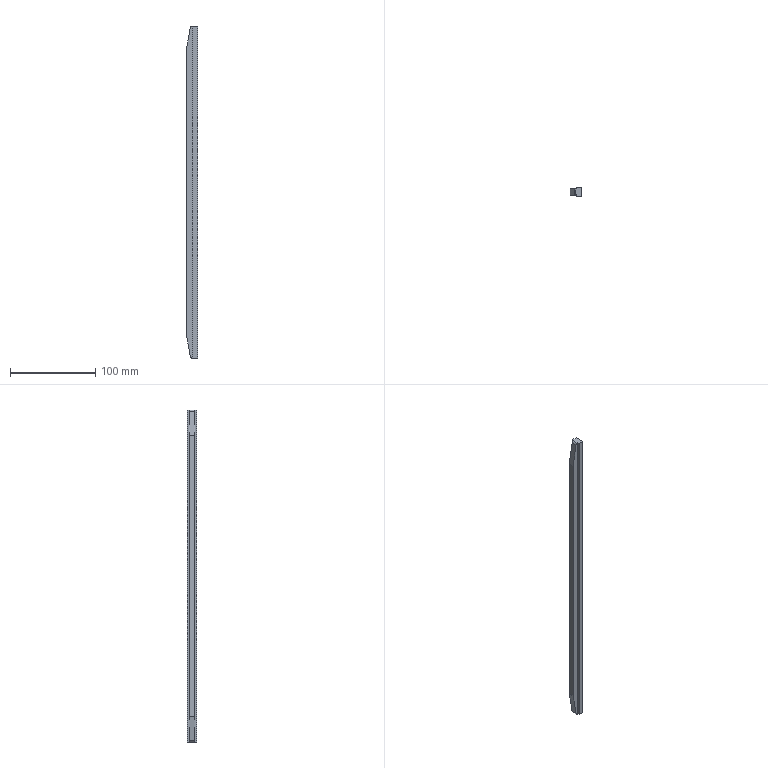Part | SolidWorks | features Chamfer 1, Extrusion 1, Fillet 1 | 1 solid | 16 faces | box 14 x 11 x 390 mm | volume 45277 mm3 | plane 12 | cylinder 4 | commonest cylinder face diameters 4 x4
STEP:
#1=CARTESIAN_POINT('',(0.,5.5,-195.));
#2=VERTEX_POINT('',#1);
#3=CARTESIAN_POINT('',(-6.,5.5,-195.));
#4=VERTEX_POINT('',#3);
#5=CARTESIAN_POINT('',(0.,5.5,-195.));
#6=DIRECTION('',(-1.,0.,0.));
#7=VECTOR('',#6,1000.);
#8=LINE('',#5,#7);
#9=EDGE_CURVE('',#2,#4,#8,.T.);
#10=ORIENTED_EDGE('',*,*,#9,.T.);
#11=CARTESIAN_POINT('',(-6.,5.5,195.));
#12=VERTEX_POINT('',#11);
#13=CARTESIAN_POINT('',(-6.,5.5,195.));
#14=DIRECTION('',(0.,0.,-1.));
#15=VECTOR('',#14,1000.);
#16=LINE('',#13,#15);
#17=EDGE_CURVE('',#12,#4,#16,.T.);
#18=ORIENTED_EDGE('',*,*,#17,.F.);
#19=CARTESIAN_POINT('',(0.,5.5,195.));
#20=VERTEX_POINT('',#19);
#21=CARTESIAN_POINT('',(0.,5.5,195.));
#22=DIRECTION('',(-1.,0.,0.));
#23=VECTOR('',#22,1000.);
#24=LINE('',#21,#23);
#25=EDGE_CURVE('',#20,#12,#24,.T.);
#26=ORIENTED_EDGE('',*,*,#25,.F.);
#27=CARTESIAN_POINT('',(0.,5.5,195.));
#28=DIRECTION('',(0.,0.,-1.));
#29=VECTOR('',#28,1000.);
#30=LINE('',#27,#29);
#31=EDGE_CURVE('',#20,#2,#30,.T.);
#32=ORIENTED_EDGE('',*,*,#31,.T.);
#33=EDGE_LOOP('',(#10,#18,#26,#32));
#34=FACE_OUTER_BOUND('',#33,.T.);
#35=CARTESIAN_POINT('',(0.,5.5,195.));
#36=DIRECTION('',(0.,-1.,0.));
#37=DIRECTION('',(1.,0.,0.));
#38=AXIS2_PLACEMENT_3D('',#35,#36,#37);
#39=PLANE('',#38);
#40=ADVANCED_FACE('',(#34),#39,.F.);
#41=CARTESIAN_POINT('',(-6.,3.3,-195.));
#42=VERTEX_POINT('',#41);
#43=CARTESIAN_POINT('',(-6.,5.5,-195.));
#44=DIRECTION('',(0.,-1.,0.));
#45=VECTOR('',#44,1000.);
#46=LINE('',#43,#45);
#47=EDGE_CURVE('',#4,#42,#46,.T.);
#48=ORIENTED_EDGE('',*,*,#47,.T.);
#49=CARTESIAN_POINT('',(-6.,3.3,195.));
#50=VERTEX_POINT('',#49);
#51=CARTESIAN_POINT('',(-6.,3.3,195.));
#52=DIRECTION('',(0.,0.,-1.));
#53=VECTOR('',#52,1000.);
#54=LINE('',#51,#53);
#55=EDGE_CURVE('',#50,#42,#54,.T.);
#56=ORIENTED_EDGE('',*,*,#55,.F.);
#57=CARTESIAN_POINT('',(-6.,5.5,195.));
#58=DIRECTION('',(0.,-1.,0.));
#59=VECTOR('',#58,1000.);
#60=LINE('',#57,#59);
#61=EDGE_CURVE('',#12,#50,#60,.T.);
#62=ORIENTED_EDGE('',*,*,#61,.F.);
#63=ORIENTED_EDGE('',*,*,#17,.T.);
#64=EDGE_LOOP('',(#48,#56,#62,#63));
#65=FACE_OUTER_BOUND('',#64,.T.);
#66=CARTESIAN_POINT('',(-6.,5.5,195.));
#67=DIRECTION('',(1.,0.,0.));
#68=DIRECTION('',(0.,0.,-1.));
#69=AXIS2_PLACEMENT_3D('',#66,#67,#68);
#70=PLANE('',#69);
#71=ADVANCED_FACE('',(#65),#70,.F.);
#72=CARTESIAN_POINT('',(-13.97,3.3,165.172));
#73=VERTEX_POINT('',#72);
#74=CARTESIAN_POINT('',(-9.002,3.3,193.347));
#75=VERTEX_POINT('',#74);
#76=CARTESIAN_POINT('',(-8.71,3.3,195.));
#77=DIRECTION('',(0.1736,0.,0.9848));
#78=VECTOR('',#77,1000.);
#79=LINE('',#76,#78);
#80=EDGE_CURVE('',#73,#75,#79,.T.);
#81=ORIENTED_EDGE('',*,*,#80,.T.);
#82=CARTESIAN_POINT('',(-7.032,3.3,195.));
#83=VERTEX_POINT('',#82);
#84=CARTESIAN_POINT('',(-7.032,3.3,193.));
#85=DIRECTION('',(0.,1.,0.));
#86=DIRECTION('',(1.,0.,0.));
#87=AXIS2_PLACEMENT_3D('',#84,#85,#86);
#88=CIRCLE('',#87,2.);
#89=EDGE_CURVE('',#75,#83,#88,.T.);
#90=ORIENTED_EDGE('',*,*,#89,.T.);
#91=CARTESIAN_POINT('',(-6.,3.3,195.));
#92=DIRECTION('',(-1.,0.,0.));
#93=VECTOR('',#92,1000.);
#94=LINE('',#91,#93);
#95=EDGE_CURVE('',#50,#83,#94,.T.);
#96=ORIENTED_EDGE('',*,*,#95,.F.);
#97=ORIENTED_EDGE('',*,*,#55,.T.);
#98=CARTESIAN_POINT('',(-7.032,3.3,-195.));
#99=VERTEX_POINT('',#98);
#100=CARTESIAN_POINT('',(-6.,3.3,-195.));
#101=DIRECTION('',(-1.,0.,0.));
#102=VECTOR('',#101,1000.);
#103=LINE('',#100,#102);
#104=EDGE_CURVE('',#42,#99,#103,.T.);
#105=ORIENTED_EDGE('',*,*,#104,.T.);
#106=CARTESIAN_POINT('',(-9.002,3.3,-193.347));
#107=VERTEX_POINT('',#106);
#108=CARTESIAN_POINT('',(-7.032,3.3,-193.));
#109=DIRECTION('',(0.,1.,0.));
#110=DIRECTION('',(1.,0.,0.));
#111=AXIS2_PLACEMENT_3D('',#108,#109,#110);
#112=CIRCLE('',#111,2.);
#113=EDGE_CURVE('',#99,#107,#112,.T.);
#114=ORIENTED_EDGE('',*,*,#113,.T.);
#115=CARTESIAN_POINT('',(-13.97,3.3,-165.172));
#116=VERTEX_POINT('',#115);
#117=CARTESIAN_POINT('',(-14.,3.3,-165.));
#118=DIRECTION('',(-0.1736,0.,0.9848));
#119=VECTOR('',#118,1000.);
#120=LINE('',#117,#119);
#121=EDGE_CURVE('',#107,#116,#120,.T.);
#122=ORIENTED_EDGE('',*,*,#121,.T.);
#123=CARTESIAN_POINT('',(-14.,3.3,-164.825));
#124=VERTEX_POINT('',#123);
#125=CARTESIAN_POINT('',(-12.,3.3,-164.825));
#126=DIRECTION('',(0.,1.,0.));
#127=DIRECTION('',(1.,0.,0.));
#128=AXIS2_PLACEMENT_3D('',#125,#126,#127);
#129=CIRCLE('',#128,2.);
#130=EDGE_CURVE('',#116,#124,#129,.T.);
#131=ORIENTED_EDGE('',*,*,#130,.T.);
#132=CARTESIAN_POINT('',(-14.,3.3,164.825));
#133=VERTEX_POINT('',#132);
#134=CARTESIAN_POINT('',(-14.,3.3,195.));
#135=DIRECTION('',(0.,0.,-1.));
#136=VECTOR('',#135,1000.);
#137=LINE('',#134,#136);
#138=EDGE_CURVE('',#133,#124,#137,.T.);
#139=ORIENTED_EDGE('',*,*,#138,.F.);
#140=CARTESIAN_POINT('',(-12.,3.3,164.825));
#141=DIRECTION('',(0.,1.,0.));
#142=DIRECTION('',(1.,0.,0.));
#143=AXIS2_PLACEMENT_3D('',#140,#141,#142);
#144=CIRCLE('',#143,2.);
#145=EDGE_CURVE('',#133,#73,#144,.T.);
#146=ORIENTED_EDGE('',*,*,#145,.T.);
#147=EDGE_LOOP('',(#81,#90,#96,#97,#105,#114,#122,#131,#139,#146));
#148=FACE_OUTER_BOUND('',#147,.T.);
#149=CARTESIAN_POINT('',(-6.,3.3,195.));
#150=DIRECTION('',(0.,-1.,0.));
#151=DIRECTION('',(1.,0.,0.));
#152=AXIS2_PLACEMENT_3D('',#149,#150,#151);
#153=PLANE('',#152);
#154=ADVANCED_FACE('',(#148),#153,.F.);
#155=CARTESIAN_POINT('',(-14.,-3.3,164.825));
#156=VERTEX_POINT('',#155);
#157=CARTESIAN_POINT('',(-14.,-3.3,-164.825));
#158=VERTEX_POINT('',#157);
#159=CARTESIAN_POINT('',(-14.,-3.3,195.));
#160=DIRECTION('',(0.,0.,-1.));
#161=VECTOR('',#160,1000.);
#162=LINE('',#159,#161);
#163=EDGE_CURVE('',#156,#158,#162,.T.);
#164=ORIENTED_EDGE('',*,*,#163,.F.);
#165=CARTESIAN_POINT('',(-14.,3.3,164.825));
#166=DIRECTION('',(0.,1.,0.));
#167=VECTOR('',#166,1000.);
#168=LINE('',#165,#167);
#169=EDGE_CURVE('',#156,#133,#168,.T.);
#170=ORIENTED_EDGE('',*,*,#169,.T.);
#171=ORIENTED_EDGE('',*,*,#138,.T.);
#172=CARTESIAN_POINT('',(-14.,-3.3,-164.825));
#173=DIRECTION('',(0.,-1.,0.));
#174=VECTOR('',#173,1000.);
#175=LINE('',#172,#174);
#176=EDGE_CURVE('',#124,#158,#175,.T.);
#177=ORIENTED_EDGE('',*,*,#176,.T.);
#178=EDGE_LOOP('',(#164,#170,#171,#177));
#179=FACE_OUTER_BOUND('',#178,.T.);
#180=CARTESIAN_POINT('',(-14.,3.3,195.));
#181=DIRECTION('',(1.,0.,0.));
#182=DIRECTION('',(0.,0.,-1.));
#183=AXIS2_PLACEMENT_3D('',#180,#181,#182);
#184=PLANE('',#183);
#185=ADVANCED_FACE('',(#179),#184,.F.);
#186=CARTESIAN_POINT('',(-7.032,-3.3,195.));
#187=VERTEX_POINT('',#186);
#188=CARTESIAN_POINT('',(-6.,-3.3,195.));
#189=VERTEX_POINT('',#188);
#190=CARTESIAN_POINT('',(-6.,-3.3,195.));
#191=DIRECTION('',(1.,0.,0.));
#192=VECTOR('',#191,1000.);
#193=LINE('',#190,#192);
#194=EDGE_CURVE('',#187,#189,#193,.T.);
#195=ORIENTED_EDGE('',*,*,#194,.F.);
#196=CARTESIAN_POINT('',(-9.002,-3.3,193.347));
#197=VERTEX_POINT('',#196);
#198=CARTESIAN_POINT('',(-7.032,-3.3,193.));
#199=DIRECTION('',(0.,-1.,0.));
#200=DIRECTION('',(-1.,0.,0.));
#201=AXIS2_PLACEMENT_3D('',#198,#199,#200);
#202=CIRCLE('',#201,2.);
#203=EDGE_CURVE('',#187,#197,#202,.T.);
#204=ORIENTED_EDGE('',*,*,#203,.T.);
#205=CARTESIAN_POINT('',(-13.97,-3.3,165.172));
#206=VERTEX_POINT('',#205);
#207=CARTESIAN_POINT('',(-8.71,-3.3,195.));
#208=DIRECTION('',(-0.1736,0.,-0.9848));
#209=VECTOR('',#208,1000.);
#210=LINE('',#207,#209);
#211=EDGE_CURVE('',#197,#206,#210,.T.);
#212=ORIENTED_EDGE('',*,*,#211,.T.);
#213=CARTESIAN_POINT('',(-12.,-3.3,164.825));
#214=DIRECTION('',(0.,-1.,0.));
#215=DIRECTION('',(-1.,0.,0.));
#216=AXIS2_PLACEMENT_3D('',#213,#214,#215);
#217=CIRCLE('',#216,2.);
#218=EDGE_CURVE('',#206,#156,#217,.T.);
#219=ORIENTED_EDGE('',*,*,#218,.T.);
#220=ORIENTED_EDGE('',*,*,#163,.T.);
#221=CARTESIAN_POINT('',(-13.97,-3.3,-165.172));
#222=VERTEX_POINT('',#221);
#223=CARTESIAN_POINT('',(-12.,-3.3,-164.825));
#224=DIRECTION('',(0.,-1.,0.));
#225=DIRECTION('',(-1.,0.,0.));
#226=AXIS2_PLACEMENT_3D('',#223,#224,#225);
#227=CIRCLE('',#226,2.);
#228=EDGE_CURVE('',#158,#222,#227,.T.);
#229=ORIENTED_EDGE('',*,*,#228,.T.);
#230=CARTESIAN_POINT('',(-9.002,-3.3,-193.347));
#231=VERTEX_POINT('',#230);
#232=CARTESIAN_POINT('',(-14.,-3.3,-165.));
#233=DIRECTION('',(0.1736,0.,-0.9848));
#234=VECTOR('',#233,1000.);
#235=LINE('',#232,#234);
#236=EDGE_CURVE('',#222,#231,#235,.T.);
#237=ORIENTED_EDGE('',*,*,#236,.T.);
#238=CARTESIAN_POINT('',(-7.032,-3.3,-195.));
#239=VERTEX_POINT('',#238);
#240=CARTESIAN_POINT('',(-7.032,-3.3,-193.));
#241=DIRECTION('',(0.,-1.,0.));
#242=DIRECTION('',(-1.,0.,0.));
#243=AXIS2_PLACEMENT_3D('',#240,#241,#242);
#244=CIRCLE('',#243,2.);
#245=EDGE_CURVE('',#231,#239,#244,.T.);
#246=ORIENTED_EDGE('',*,*,#245,.T.);
#247=CARTESIAN_POINT('',(-6.,-3.3,-195.));
#248=VERTEX_POINT('',#247);
#249=CARTESIAN_POINT('',(-6.,-3.3,-195.));
#250=DIRECTION('',(1.,0.,0.));
#251=VECTOR('',#250,1000.);
#252=LINE('',#249,#251);
#253=EDGE_CURVE('',#239,#248,#252,.T.);
#254=ORIENTED_EDGE('',*,*,#253,.T.);
#255=CARTESIAN_POINT('',(-6.,-3.3,195.));
#256=DIRECTION('',(0.,0.,-1.));
#257=VECTOR('',#256,1000.);
#258=LINE('',#255,#257);
#259=EDGE_CURVE('',#189,#248,#258,.T.);
#260=ORIENTED_EDGE('',*,*,#259,.F.);
#261=EDGE_LOOP('',(#195,#204,#212,#219,#220,#229,#237,#246,#254,#260));
#262=FACE_OUTER_BOUND('',#261,.T.);
#263=CARTESIAN_POINT('',(-6.,-3.3,195.));
#264=DIRECTION('',(0.,1.,0.));
#265=DIRECTION('',(-1.,0.,0.));
#266=AXIS2_PLACEMENT_3D('',#263,#264,#265);
#267=PLANE('',#266);
#268=ADVANCED_FACE('',(#262),#267,.F.);
#269=CARTESIAN_POINT('',(-6.,-5.5,-195.));
#270=VERTEX_POINT('',#269);
#271=CARTESIAN_POINT('',(-6.,-5.5,-195.));
#272=DIRECTION('',(0.,-1.,0.));
#273=VECTOR('',#272,1000.);
#274=LINE('',#271,#273);
#275=EDGE_CURVE('',#248,#270,#274,.T.);
#276=ORIENTED_EDGE('',*,*,#275,.T.);
#277=CARTESIAN_POINT('',(-6.,-5.5,195.));
#278=VERTEX_POINT('',#277);
#279=CARTESIAN_POINT('',(-6.,-5.5,195.));
#280=DIRECTION('',(0.,0.,-1.));
#281=VECTOR('',#280,1000.);
#282=LINE('',#279,#281);
#283=EDGE_CURVE('',#278,#270,#282,.T.);
#284=ORIENTED_EDGE('',*,*,#283,.F.);
#285=CARTESIAN_POINT('',(-6.,-5.5,195.));
#286=DIRECTION('',(0.,-1.,0.));
#287=VECTOR('',#286,1000.);
#288=LINE('',#285,#287);
#289=EDGE_CURVE('',#189,#278,#288,.T.);
#290=ORIENTED_EDGE('',*,*,#289,.F.);
#291=ORIENTED_EDGE('',*,*,#259,.T.);
#292=EDGE_LOOP('',(#276,#284,#290,#291));
#293=FACE_OUTER_BOUND('',#292,.T.);
#294=CARTESIAN_POINT('',(-6.,-5.5,195.));
#295=DIRECTION('',(1.,0.,0.));
#296=DIRECTION('',(0.,0.,-1.));
#297=AXIS2_PLACEMENT_3D('',#294,#295,#296);
#298=PLANE('',#297);
#299=ADVANCED_FACE('',(#293),#298,.F.);
#300=CARTESIAN_POINT('',(0.,-5.5,-195.));
#301=VERTEX_POINT('',#300);
#302=CARTESIAN_POINT('',(0.,-5.5,-195.));
#303=DIRECTION('',(1.,0.,0.));
#304=VECTOR('',#303,1000.);
#305=LINE('',#302,#304);
#306=EDGE_CURVE('',#270,#301,#305,.T.);
#307=ORIENTED_EDGE('',*,*,#306,.T.);
#308=CARTESIAN_POINT('',(0.,-5.5,195.));
#309=VERTEX_POINT('',#308);
#310=CARTESIAN_POINT('',(0.,-5.5,195.));
#311=DIRECTION('',(0.,0.,-1.));
#312=VECTOR('',#311,1000.);
#313=LINE('',#310,#312);
#314=EDGE_CURVE('',#309,#301,#313,.T.);
#315=ORIENTED_EDGE('',*,*,#314,.F.);
#316=CARTESIAN_POINT('',(0.,-5.5,195.));
#317=DIRECTION('',(1.,0.,0.));
#318=VECTOR('',#317,1000.);
#319=LINE('',#316,#318);
#320=EDGE_CURVE('',#278,#309,#319,.T.);
#321=ORIENTED_EDGE('',*,*,#320,.F.);
#322=ORIENTED_EDGE('',*,*,#283,.T.);
#323=EDGE_LOOP('',(#307,#315,#321,#322));
#324=FACE_OUTER_BOUND('',#323,.T.);
#325=CARTESIAN_POINT('',(0.,-5.5,195.));
#326=DIRECTION('',(0.,1.,0.));
#327=DIRECTION('',(-1.,0.,0.));
#328=AXIS2_PLACEMENT_3D('',#325,#326,#327);
#329=PLANE('',#328);
#330=ADVANCED_FACE('',(#324),#329,.F.);
#331=CARTESIAN_POINT('',(0.,-5.5,-195.));
#332=DIRECTION('',(0.,1.,0.));
#333=VECTOR('',#332,1000.);
#334=LINE('',#331,#333);
#335=EDGE_CURVE('',#301,#2,#334,.T.);
#336=ORIENTED_EDGE('',*,*,#335,.T.);
#337=ORIENTED_EDGE('',*,*,#31,.F.);
#338=CARTESIAN_POINT('',(0.,-5.5,195.));
#339=DIRECTION('',(0.,1.,0.));
#340=VECTOR('',#339,1000.);
#341=LINE('',#338,#340);
#342=EDGE_CURVE('',#309,#20,#341,.T.);
#343=ORIENTED_EDGE('',*,*,#342,.F.);
#344=ORIENTED_EDGE('',*,*,#314,.T.);
#345=EDGE_LOOP('',(#336,#337,#343,#344));
#346=FACE_OUTER_BOUND('',#345,.T.);
#347=CARTESIAN_POINT('',(0.,-5.5,195.));
#348=DIRECTION('',(-1.,0.,0.));
#349=DIRECTION('',(0.,0.,1.));
#350=AXIS2_PLACEMENT_3D('',#347,#348,#349);
#351=PLANE('',#350);
#352=ADVANCED_FACE('',(#346),#351,.F.);
#353=ORIENTED_EDGE('',*,*,#95,.T.);
#354=CARTESIAN_POINT('',(-7.032,0.,195.));
#355=DIRECTION('',(0.,-1.,0.));
#356=VECTOR('',#355,1000.);
#357=LINE('',#354,#356);
#358=EDGE_CURVE('',#83,#187,#357,.T.);
#359=ORIENTED_EDGE('',*,*,#358,.T.);
#360=ORIENTED_EDGE('',*,*,#194,.T.);
#361=ORIENTED_EDGE('',*,*,#289,.T.);
#362=ORIENTED_EDGE('',*,*,#320,.T.);
#363=ORIENTED_EDGE('',*,*,#342,.T.);
#364=ORIENTED_EDGE('',*,*,#25,.T.);
#365=ORIENTED_EDGE('',*,*,#61,.T.);
#366=EDGE_LOOP('',(#353,#359,#360,#361,#362,#363,#364,#365));
#367=FACE_OUTER_BOUND('',#366,.T.);
#368=CARTESIAN_POINT('',(0.,0.,195.));
#369=DIRECTION('',(0.,0.,1.));
#370=DIRECTION('',(1.,0.,0.));
#371=AXIS2_PLACEMENT_3D('',#368,#369,#370);
#372=PLANE('',#371);
#373=ADVANCED_FACE('',(#367),#372,.T.);
#374=ORIENTED_EDGE('',*,*,#253,.F.);
#375=CARTESIAN_POINT('',(-7.032,3.3,-195.));
#376=DIRECTION('',(0.,1.,0.));
#377=VECTOR('',#376,1000.);
#378=LINE('',#375,#377);
#379=EDGE_CURVE('',#239,#99,#378,.T.);
#380=ORIENTED_EDGE('',*,*,#379,.T.);
#381=ORIENTED_EDGE('',*,*,#104,.F.);
#382=ORIENTED_EDGE('',*,*,#47,.F.);
#383=ORIENTED_EDGE('',*,*,#9,.F.);
#384=ORIENTED_EDGE('',*,*,#335,.F.);
#385=ORIENTED_EDGE('',*,*,#306,.F.);
#386=ORIENTED_EDGE('',*,*,#275,.F.);
#387=EDGE_LOOP('',(#374,#380,#381,#382,#383,#384,#385,#386));
#388=FACE_OUTER_BOUND('',#387,.T.);
#389=CARTESIAN_POINT('',(0.,0.,-195.));
#390=DIRECTION('',(0.,0.,1.));
#391=DIRECTION('',(1.,0.,0.));
#392=AXIS2_PLACEMENT_3D('',#389,#390,#391);
#393=PLANE('',#392);
#394=ADVANCED_FACE('',(#388),#393,.F.);
#395=ORIENTED_EDGE('',*,*,#236,.F.);
#396=CARTESIAN_POINT('',(-13.97,3.3,-165.172));
#397=DIRECTION('',(0.,1.,0.));
#398=VECTOR('',#397,1000.);
#399=LINE('',#396,#398);
#400=EDGE_CURVE('',#222,#116,#399,.T.);
#401=ORIENTED_EDGE('',*,*,#400,.T.);
#402=ORIENTED_EDGE('',*,*,#121,.F.);
#403=CARTESIAN_POINT('',(-9.002,-3.3,-193.347));
#404=DIRECTION('',(0.,-1.,0.));
#405=VECTOR('',#404,1000.);
#406=LINE('',#403,#405);
#407=EDGE_CURVE('',#107,#231,#406,.T.);
#408=ORIENTED_EDGE('',*,*,#407,.T.);
#409=EDGE_LOOP('',(#395,#401,#402,#408));
#410=FACE_OUTER_BOUND('',#409,.T.);
#411=CARTESIAN_POINT('',(-14.,3.3,-165.));
#412=DIRECTION('',(0.9848,0.,0.1736));
#413=DIRECTION('',(0.,-1.,0.));
#414=AXIS2_PLACEMENT_3D('',#411,#412,#413);
#415=PLANE('',#414);
#416=ADVANCED_FACE('',(#410),#415,.F.);
#417=ORIENTED_EDGE('',*,*,#211,.F.);
#418=CARTESIAN_POINT('',(-9.002,0.,193.347));
#419=DIRECTION('',(0.,1.,0.));
#420=VECTOR('',#419,1000.);
#421=LINE('',#418,#420);
#422=EDGE_CURVE('',#197,#75,#421,.T.);
#423=ORIENTED_EDGE('',*,*,#422,.T.);
#424=ORIENTED_EDGE('',*,*,#80,.F.);
#425=CARTESIAN_POINT('',(-13.97,-3.3,165.172));
#426=DIRECTION('',(0.,-1.,0.));
#427=VECTOR('',#426,1000.);
#428=LINE('',#425,#427);
#429=EDGE_CURVE('',#73,#206,#428,.T.);
#430=ORIENTED_EDGE('',*,*,#429,.T.);
#431=EDGE_LOOP('',(#417,#423,#424,#430));
#432=FACE_OUTER_BOUND('',#431,.T.);
#433=CARTESIAN_POINT('',(-8.71,0.,195.));
#434=DIRECTION('',(-0.9848,0.,0.1736));
#435=DIRECTION('',(0.,1.,0.));
#436=AXIS2_PLACEMENT_3D('',#433,#434,#435);
#437=PLANE('',#436);
#438=ADVANCED_FACE('',(#432),#437,.T.);
#439=ORIENTED_EDGE('',*,*,#89,.F.);
#440=ORIENTED_EDGE('',*,*,#422,.F.);
#441=ORIENTED_EDGE('',*,*,#203,.F.);
#442=ORIENTED_EDGE('',*,*,#358,.F.);
#443=EDGE_LOOP('',(#439,#440,#441,#442));
#444=FACE_OUTER_BOUND('',#443,.T.);
#445=CARTESIAN_POINT('',(-7.032,0.,193.));
#446=DIRECTION('',(0.,-1.,0.));
#447=DIRECTION('',(0.,0.,-1.));
#448=AXIS2_PLACEMENT_3D('',#445,#446,#447);
#449=CYLINDRICAL_SURFACE('',#448,2.);
#450=ADVANCED_FACE('',(#444),#449,.T.);
#451=ORIENTED_EDGE('',*,*,#218,.F.);
#452=ORIENTED_EDGE('',*,*,#429,.F.);
#453=ORIENTED_EDGE('',*,*,#145,.F.);
#454=ORIENTED_EDGE('',*,*,#169,.F.);
#455=EDGE_LOOP('',(#451,#452,#453,#454));
#456=FACE_OUTER_BOUND('',#455,.T.);
#457=CARTESIAN_POINT('',(-12.,3.3,164.825));
#458=DIRECTION('',(0.,-1.,0.));
#459=DIRECTION('',(0.,0.,-1.));
#460=AXIS2_PLACEMENT_3D('',#457,#458,#459);
#461=CYLINDRICAL_SURFACE('',#460,2.);
#462=ADVANCED_FACE('',(#456),#461,.T.);
#463=ORIENTED_EDGE('',*,*,#130,.F.);
#464=ORIENTED_EDGE('',*,*,#400,.F.);
#465=ORIENTED_EDGE('',*,*,#228,.F.);
#466=ORIENTED_EDGE('',*,*,#176,.F.);
#467=EDGE_LOOP('',(#463,#464,#465,#466));
#468=FACE_OUTER_BOUND('',#467,.T.);
#469=CARTESIAN_POINT('',(-12.,3.3,-164.825));
#470=DIRECTION('',(0.,-1.,0.));
#471=DIRECTION('',(0.,0.,-1.));
#472=AXIS2_PLACEMENT_3D('',#469,#470,#471);
#473=CYLINDRICAL_SURFACE('',#472,2.);
#474=ADVANCED_FACE('',(#468),#473,.T.);
#475=ORIENTED_EDGE('',*,*,#245,.F.);
#476=ORIENTED_EDGE('',*,*,#407,.F.);
#477=ORIENTED_EDGE('',*,*,#113,.F.);
#478=ORIENTED_EDGE('',*,*,#379,.F.);
#479=EDGE_LOOP('',(#475,#476,#477,#478));
#480=FACE_OUTER_BOUND('',#479,.T.);
#481=CARTESIAN_POINT('',(-7.032,0.,-193.));
#482=DIRECTION('',(0.,1.,0.));
#483=DIRECTION('',(0.,0.,1.));
#484=AXIS2_PLACEMENT_3D('',#481,#482,#483);
#485=CYLINDRICAL_SURFACE('',#484,2.);
#486=ADVANCED_FACE('',(#480),#485,.T.);
#487=CLOSED_SHELL('',(#40,#71,#154,#185,#268,#299,#330,#352,#373,#394,#416,#438,#450,#462,#474,#486));
#488=MANIFOLD_SOLID_BREP('',#487);
#489=CARTESIAN_POINT('',(0.,0.,0.));
#490=DIRECTION('',(0.,0.,1.));
#491=DIRECTION('',(1.,0.,0.));
#492=AXIS2_PLACEMENT_3D('',#489,#490,#491);
#493=(LENGTH_UNIT()NAMED_UNIT(*)SI_UNIT(.MILLI.,.METRE.));
#494=UNCERTAINTY_MEASURE_WITH_UNIT(LENGTH_MEASURE(0.00001),#493,'','');
#495=(NAMED_UNIT(*)PLANE_ANGLE_UNIT()SI_UNIT($,.RADIAN.));
#496=(NAMED_UNIT(*)SI_UNIT($,.STERADIAN.)SOLID_ANGLE_UNIT());
#497=(GEOMETRIC_REPRESENTATION_CONTEXT(3)GLOBAL_UNCERTAINTY_ASSIGNED_CONTEXT((#494))GLOBAL_UNIT_ASSIGNED_CONTEXT((#493,#495,#496))REPRESENTATION_CONTEXT('',''));
#498=ADVANCED_BREP_SHAPE_REPRESENTATION('',(#488,#492),#497);